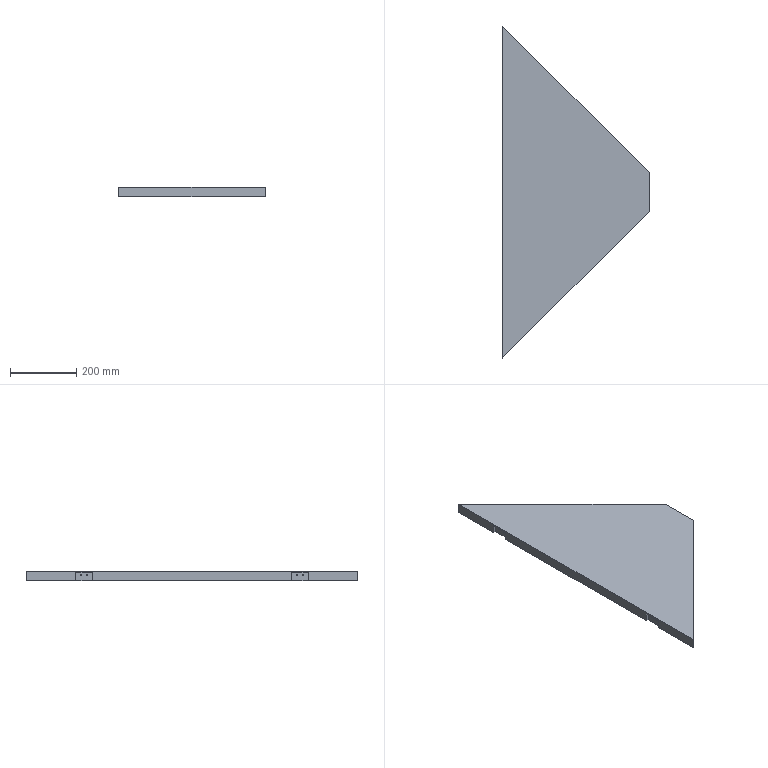Part | SolidWorks | features Cut 1, Extrusion 1, HoleWzd 1, ICE 1, Shell 1 | 1 solid | 35 faces | box 440 x 1000 x 30 mm | volume 2685666 mm3 | plane 27 | cylinder 8 | commonest cylinder face diameters 3.3 x8
STEP:
#1=CARTESIAN_POINT('',(-488.,335.,19.15));
#2=VERTEX_POINT('',#1);
#3=CARTESIAN_POINT('',(-488.,335.,15.85));
#4=VERTEX_POINT('',#3);
#5=CARTESIAN_POINT('',(-488.,335.,17.5));
#6=DIRECTION('',(1.,0.,0.));
#7=DIRECTION('',(0.,0.,-1.));
#8=AXIS2_PLACEMENT_3D('',#5,#6,#7);
#9=CIRCLE('',#8,1.65);
#10=EDGE_CURVE('',#2,#4,#9,.T.);
#11=ORIENTED_EDGE('',*,*,#10,.T.);
#12=CARTESIAN_POINT('',(-493.,335.,15.85));
#13=VERTEX_POINT('',#12);
#14=CARTESIAN_POINT('',(-493.,335.,15.85));
#15=DIRECTION('',(-1.,0.,0.));
#16=VECTOR('',#15,1000.);
#17=LINE('',#14,#16);
#18=EDGE_CURVE('',#4,#13,#17,.T.);
#19=ORIENTED_EDGE('',*,*,#18,.T.);
#20=CARTESIAN_POINT('',(-493.,335.,19.15));
#21=VERTEX_POINT('',#20);
#22=CARTESIAN_POINT('',(-493.,335.,17.5));
#23=DIRECTION('',(-1.,0.,0.));
#24=DIRECTION('',(0.,0.,1.));
#25=AXIS2_PLACEMENT_3D('',#22,#23,#24);
#26=CIRCLE('',#25,1.65);
#27=EDGE_CURVE('',#13,#21,#26,.T.);
#28=ORIENTED_EDGE('',*,*,#27,.T.);
#29=CARTESIAN_POINT('',(-493.,335.,19.15));
#30=DIRECTION('',(-1.,0.,0.));
#31=VECTOR('',#30,1000.);
#32=LINE('',#29,#31);
#33=EDGE_CURVE('',#2,#21,#32,.T.);
#34=ORIENTED_EDGE('',*,*,#33,.F.);
#35=EDGE_LOOP('',(#11,#19,#28,#34));
#36=FACE_OUTER_BOUND('',#35,.T.);
#37=CARTESIAN_POINT('',(-493.,335.,17.5));
#38=DIRECTION('',(-1.,0.,0.));
#39=DIRECTION('',(0.,0.,1.));
#40=AXIS2_PLACEMENT_3D('',#37,#38,#39);
#41=CYLINDRICAL_SURFACE('',#40,1.65);
#42=ADVANCED_FACE('',(#36),#41,.F.);
#43=CARTESIAN_POINT('',(-488.,315.,19.15));
#44=VERTEX_POINT('',#43);
#45=CARTESIAN_POINT('',(-488.,315.,15.85));
#46=VERTEX_POINT('',#45);
#47=CARTESIAN_POINT('',(-488.,315.,17.5));
#48=DIRECTION('',(1.,0.,0.));
#49=DIRECTION('',(0.,0.,-1.));
#50=AXIS2_PLACEMENT_3D('',#47,#48,#49);
#51=CIRCLE('',#50,1.65);
#52=EDGE_CURVE('',#44,#46,#51,.T.);
#53=ORIENTED_EDGE('',*,*,#52,.T.);
#54=CARTESIAN_POINT('',(-493.,315.,15.85));
#55=VERTEX_POINT('',#54);
#56=CARTESIAN_POINT('',(-493.,315.,15.85));
#57=DIRECTION('',(-1.,0.,0.));
#58=VECTOR('',#57,1000.);
#59=LINE('',#56,#58);
#60=EDGE_CURVE('',#46,#55,#59,.T.);
#61=ORIENTED_EDGE('',*,*,#60,.T.);
#62=CARTESIAN_POINT('',(-493.,315.,19.15));
#63=VERTEX_POINT('',#62);
#64=CARTESIAN_POINT('',(-493.,315.,17.5));
#65=DIRECTION('',(-1.,0.,0.));
#66=DIRECTION('',(0.,0.,1.));
#67=AXIS2_PLACEMENT_3D('',#64,#65,#66);
#68=CIRCLE('',#67,1.65);
#69=EDGE_CURVE('',#55,#63,#68,.T.);
#70=ORIENTED_EDGE('',*,*,#69,.T.);
#71=CARTESIAN_POINT('',(-493.,315.,19.15));
#72=DIRECTION('',(-1.,0.,0.));
#73=VECTOR('',#72,1000.);
#74=LINE('',#71,#73);
#75=EDGE_CURVE('',#44,#63,#74,.T.);
#76=ORIENTED_EDGE('',*,*,#75,.F.);
#77=EDGE_LOOP('',(#53,#61,#70,#76));
#78=FACE_OUTER_BOUND('',#77,.T.);
#79=CARTESIAN_POINT('',(-493.,315.,17.5));
#80=DIRECTION('',(-1.,0.,0.));
#81=DIRECTION('',(0.,0.,1.));
#82=AXIS2_PLACEMENT_3D('',#79,#80,#81);
#83=CYLINDRICAL_SURFACE('',#82,1.65);
#84=ADVANCED_FACE('',(#78),#83,.F.);
#85=CARTESIAN_POINT('',(-488.,-315.,19.15));
#86=VERTEX_POINT('',#85);
#87=CARTESIAN_POINT('',(-488.,-315.,15.85));
#88=VERTEX_POINT('',#87);
#89=CARTESIAN_POINT('',(-488.,-315.,17.5));
#90=DIRECTION('',(1.,0.,0.));
#91=DIRECTION('',(0.,0.,-1.));
#92=AXIS2_PLACEMENT_3D('',#89,#90,#91);
#93=CIRCLE('',#92,1.65);
#94=EDGE_CURVE('',#86,#88,#93,.T.);
#95=ORIENTED_EDGE('',*,*,#94,.T.);
#96=CARTESIAN_POINT('',(-493.,-315.,15.85));
#97=VERTEX_POINT('',#96);
#98=CARTESIAN_POINT('',(-493.,-315.,15.85));
#99=DIRECTION('',(-1.,0.,0.));
#100=VECTOR('',#99,1000.);
#101=LINE('',#98,#100);
#102=EDGE_CURVE('',#88,#97,#101,.T.);
#103=ORIENTED_EDGE('',*,*,#102,.T.);
#104=CARTESIAN_POINT('',(-493.,-315.,19.15));
#105=VERTEX_POINT('',#104);
#106=CARTESIAN_POINT('',(-493.,-315.,17.5));
#107=DIRECTION('',(-1.,0.,0.));
#108=DIRECTION('',(0.,0.,1.));
#109=AXIS2_PLACEMENT_3D('',#106,#107,#108);
#110=CIRCLE('',#109,1.65);
#111=EDGE_CURVE('',#97,#105,#110,.T.);
#112=ORIENTED_EDGE('',*,*,#111,.T.);
#113=CARTESIAN_POINT('',(-493.,-315.,19.15));
#114=DIRECTION('',(-1.,0.,0.));
#115=VECTOR('',#114,1000.);
#116=LINE('',#113,#115);
#117=EDGE_CURVE('',#86,#105,#116,.T.);
#118=ORIENTED_EDGE('',*,*,#117,.F.);
#119=EDGE_LOOP('',(#95,#103,#112,#118));
#120=FACE_OUTER_BOUND('',#119,.T.);
#121=CARTESIAN_POINT('',(-493.,-315.,17.5));
#122=DIRECTION('',(-1.,0.,0.));
#123=DIRECTION('',(0.,0.,1.));
#124=AXIS2_PLACEMENT_3D('',#121,#122,#123);
#125=CYLINDRICAL_SURFACE('',#124,1.65);
#126=ADVANCED_FACE('',(#120),#125,.F.);
#127=CARTESIAN_POINT('',(-488.,-335.,19.15));
#128=VERTEX_POINT('',#127);
#129=CARTESIAN_POINT('',(-488.,-335.,15.85));
#130=VERTEX_POINT('',#129);
#131=CARTESIAN_POINT('',(-488.,-335.,17.5));
#132=DIRECTION('',(1.,0.,0.));
#133=DIRECTION('',(0.,0.,-1.));
#134=AXIS2_PLACEMENT_3D('',#131,#132,#133);
#135=CIRCLE('',#134,1.65);
#136=EDGE_CURVE('',#128,#130,#135,.T.);
#137=ORIENTED_EDGE('',*,*,#136,.T.);
#138=CARTESIAN_POINT('',(-493.,-335.,15.85));
#139=VERTEX_POINT('',#138);
#140=CARTESIAN_POINT('',(-493.,-335.,15.85));
#141=DIRECTION('',(-1.,0.,0.));
#142=VECTOR('',#141,1000.);
#143=LINE('',#140,#142);
#144=EDGE_CURVE('',#130,#139,#143,.T.);
#145=ORIENTED_EDGE('',*,*,#144,.T.);
#146=CARTESIAN_POINT('',(-493.,-335.,19.15));
#147=VERTEX_POINT('',#146);
#148=CARTESIAN_POINT('',(-493.,-335.,17.5));
#149=DIRECTION('',(-1.,0.,0.));
#150=DIRECTION('',(0.,0.,1.));
#151=AXIS2_PLACEMENT_3D('',#148,#149,#150);
#152=CIRCLE('',#151,1.65);
#153=EDGE_CURVE('',#139,#147,#152,.T.);
#154=ORIENTED_EDGE('',*,*,#153,.T.);
#155=CARTESIAN_POINT('',(-493.,-335.,19.15));
#156=DIRECTION('',(-1.,0.,0.));
#157=VECTOR('',#156,1000.);
#158=LINE('',#155,#157);
#159=EDGE_CURVE('',#128,#147,#158,.T.);
#160=ORIENTED_EDGE('',*,*,#159,.F.);
#161=EDGE_LOOP('',(#137,#145,#154,#160));
#162=FACE_OUTER_BOUND('',#161,.T.);
#163=CARTESIAN_POINT('',(-493.,-335.,17.5));
#164=DIRECTION('',(-1.,0.,0.));
#165=DIRECTION('',(0.,0.,1.));
#166=AXIS2_PLACEMENT_3D('',#163,#164,#165);
#167=CYLINDRICAL_SURFACE('',#166,1.65);
#168=ADVANCED_FACE('',(#162),#167,.F.);
#169=CARTESIAN_POINT('',(-60.,60.,30.));
#170=VERTEX_POINT('',#169);
#171=CARTESIAN_POINT('',(-60.,-60.,30.));
#172=VERTEX_POINT('',#171);
#173=CARTESIAN_POINT('',(-60.,-60.,30.));
#174=DIRECTION('',(0.,-1.,0.));
#175=VECTOR('',#174,1000.);
#176=LINE('',#173,#175);
#177=EDGE_CURVE('',#170,#172,#176,.T.);
#178=ORIENTED_EDGE('',*,*,#177,.T.);
#179=CARTESIAN_POINT('',(-60.,-60.,0.));
#180=VERTEX_POINT('',#179);
#181=CARTESIAN_POINT('',(-60.,-60.,0.));
#182=DIRECTION('',(0.,0.,1.));
#183=VECTOR('',#182,1000.);
#184=LINE('',#181,#183);
#185=EDGE_CURVE('',#180,#172,#184,.T.);
#186=ORIENTED_EDGE('',*,*,#185,.F.);
#187=CARTESIAN_POINT('',(-60.,60.,0.));
#188=VERTEX_POINT('',#187);
#189=CARTESIAN_POINT('',(-60.,-60.,0.));
#190=DIRECTION('',(0.,-1.,0.));
#191=VECTOR('',#190,1000.);
#192=LINE('',#189,#191);
#193=EDGE_CURVE('',#188,#180,#192,.T.);
#194=ORIENTED_EDGE('',*,*,#193,.F.);
#195=CARTESIAN_POINT('',(-60.,60.,0.));
#196=DIRECTION('',(0.,0.,1.));
#197=VECTOR('',#196,1000.);
#198=LINE('',#195,#197);
#199=EDGE_CURVE('',#188,#170,#198,.T.);
#200=ORIENTED_EDGE('',*,*,#199,.T.);
#201=EDGE_LOOP('',(#178,#186,#194,#200));
#202=FACE_OUTER_BOUND('',#201,.T.);
#203=CARTESIAN_POINT('',(-60.,52.929,25.));
#204=VERTEX_POINT('',#203);
#205=CARTESIAN_POINT('',(-60.,-52.929,25.));
#206=VERTEX_POINT('',#205);
#207=CARTESIAN_POINT('',(-60.,0.,25.));
#208=DIRECTION('',(0.,-1.,0.));
#209=VECTOR('',#208,1000.);
#210=LINE('',#207,#209);
#211=EDGE_CURVE('',#204,#206,#210,.T.);
#212=ORIENTED_EDGE('',*,*,#211,.F.);
#213=CARTESIAN_POINT('',(-60.,52.929,5.));
#214=VERTEX_POINT('',#213);
#215=CARTESIAN_POINT('',(-60.,52.929,0.));
#216=DIRECTION('',(0.,0.,1.));
#217=VECTOR('',#216,1000.);
#218=LINE('',#215,#217);
#219=EDGE_CURVE('',#214,#204,#218,.T.);
#220=ORIENTED_EDGE('',*,*,#219,.F.);
#221=CARTESIAN_POINT('',(-60.,-52.929,5.));
#222=VERTEX_POINT('',#221);
#223=CARTESIAN_POINT('',(-60.,0.,5.));
#224=DIRECTION('',(0.,-1.,0.));
#225=VECTOR('',#224,1000.);
#226=LINE('',#223,#225);
#227=EDGE_CURVE('',#214,#222,#226,.T.);
#228=ORIENTED_EDGE('',*,*,#227,.T.);
#229=CARTESIAN_POINT('',(-60.,-52.929,30.));
#230=DIRECTION('',(0.,0.,1.));
#231=VECTOR('',#230,1000.);
#232=LINE('',#229,#231);
#233=EDGE_CURVE('',#222,#206,#232,.T.);
#234=ORIENTED_EDGE('',*,*,#233,.T.);
#235=EDGE_LOOP('',(#212,#220,#228,#234));
#236=FACE_BOUND('',#235,.T.);
#237=CARTESIAN_POINT('',(-60.,-60.,0.));
#238=DIRECTION('',(-1.,0.,0.));
#239=DIRECTION('',(0.,0.,1.));
#240=AXIS2_PLACEMENT_3D('',#237,#238,#239);
#241=PLANE('',#240);
#242=ADVANCED_FACE('',(#202,#236),#241,.F.);
#243=CARTESIAN_POINT('',(-500.,-500.,0.));
#244=VERTEX_POINT('',#243);
#245=CARTESIAN_POINT('',(0.,0.,0.));
#246=DIRECTION('',(0.7071,0.7071,0.));
#247=VECTOR('',#246,1000.);
#248=LINE('',#245,#247);
#249=EDGE_CURVE('',#244,#180,#248,.T.);
#250=ORIENTED_EDGE('',*,*,#249,.T.);
#251=ORIENTED_EDGE('',*,*,#185,.T.);
#252=CARTESIAN_POINT('',(-500.,-500.,30.));
#253=VERTEX_POINT('',#252);
#254=CARTESIAN_POINT('',(0.,0.,30.));
#255=DIRECTION('',(0.7071,0.7071,0.));
#256=VECTOR('',#255,1000.);
#257=LINE('',#254,#256);
#258=EDGE_CURVE('',#253,#172,#257,.T.);
#259=ORIENTED_EDGE('',*,*,#258,.F.);
#260=CARTESIAN_POINT('',(-500.,-500.,30.));
#261=DIRECTION('',(0.,0.,-1.));
#262=VECTOR('',#261,1000.);
#263=LINE('',#260,#262);
#264=EDGE_CURVE('',#253,#244,#263,.T.);
#265=ORIENTED_EDGE('',*,*,#264,.T.);
#266=EDGE_LOOP('',(#250,#251,#259,#265));
#267=FACE_OUTER_BOUND('',#266,.T.);
#268=CARTESIAN_POINT('',(0.,0.,30.));
#269=DIRECTION('',(-0.7071,0.7071,0.));
#270=DIRECTION('',(-0.7071,-0.7071,0.));
#271=AXIS2_PLACEMENT_3D('',#268,#269,#270);
#272=PLANE('',#271);
#273=ADVANCED_FACE('',(#267),#272,.F.);
#274=CARTESIAN_POINT('',(-500.,500.,30.));
#275=VERTEX_POINT('',#274);
#276=CARTESIAN_POINT('',(-500.,500.,30.));
#277=DIRECTION('',(-0.7071,0.7071,0.));
#278=VECTOR('',#277,1000.);
#279=LINE('',#276,#278);
#280=EDGE_CURVE('',#170,#275,#279,.T.);
#281=ORIENTED_EDGE('',*,*,#280,.F.);
#282=ORIENTED_EDGE('',*,*,#199,.F.);
#283=CARTESIAN_POINT('',(-500.,500.,0.));
#284=VERTEX_POINT('',#283);
#285=CARTESIAN_POINT('',(-500.,500.,0.));
#286=DIRECTION('',(-0.7071,0.7071,0.));
#287=VECTOR('',#286,1000.);
#288=LINE('',#285,#287);
#289=EDGE_CURVE('',#188,#284,#288,.T.);
#290=ORIENTED_EDGE('',*,*,#289,.T.);
#291=CARTESIAN_POINT('',(-500.,500.,30.));
#292=DIRECTION('',(0.,0.,-1.));
#293=VECTOR('',#292,1000.);
#294=LINE('',#291,#293);
#295=EDGE_CURVE('',#275,#284,#294,.T.);
#296=ORIENTED_EDGE('',*,*,#295,.F.);
#297=EDGE_LOOP('',(#281,#282,#290,#296));
#298=FACE_OUTER_BOUND('',#297,.T.);
#299=CARTESIAN_POINT('',(-500.,500.,30.));
#300=DIRECTION('',(-0.7071,-0.7071,0.));
#301=DIRECTION('',(0.7071,-0.7071,0.));
#302=AXIS2_PLACEMENT_3D('',#299,#300,#301);
#303=PLANE('',#302);
#304=ADVANCED_FACE('',(#298),#303,.F.);
#305=CARTESIAN_POINT('',(-500.,300.,25.));
#306=VERTEX_POINT('',#305);
#307=CARTESIAN_POINT('',(-500.,350.,25.));
#308=VERTEX_POINT('',#307);
#309=CARTESIAN_POINT('',(-500.,350.,25.));
#310=DIRECTION('',(0.,1.,0.));
#311=VECTOR('',#310,1000.);
#312=LINE('',#309,#311);
#313=EDGE_CURVE('',#306,#308,#312,.T.);
#314=ORIENTED_EDGE('',*,*,#313,.F.);
#315=CARTESIAN_POINT('',(-500.,300.,0.));
#316=VERTEX_POINT('',#315);
#317=CARTESIAN_POINT('',(-500.,300.,25.));
#318=DIRECTION('',(0.,0.,1.));
#319=VECTOR('',#318,1000.);
#320=LINE('',#317,#319);
#321=EDGE_CURVE('',#316,#306,#320,.T.);
#322=ORIENTED_EDGE('',*,*,#321,.F.);
#323=CARTESIAN_POINT('',(-500.,-300.,0.));
#324=VERTEX_POINT('',#323);
#325=CARTESIAN_POINT('',(-500.,-500.,0.));
#326=DIRECTION('',(0.,-1.,0.));
#327=VECTOR('',#326,1000.);
#328=LINE('',#325,#327);
#329=EDGE_CURVE('',#316,#324,#328,.T.);
#330=ORIENTED_EDGE('',*,*,#329,.T.);
#331=CARTESIAN_POINT('',(-500.,-300.,25.));
#332=VERTEX_POINT('',#331);
#333=CARTESIAN_POINT('',(-500.,-300.,25.));
#334=DIRECTION('',(0.,0.,-1.));
#335=VECTOR('',#334,1000.);
#336=LINE('',#333,#335);
#337=EDGE_CURVE('',#332,#324,#336,.T.);
#338=ORIENTED_EDGE('',*,*,#337,.F.);
#339=CARTESIAN_POINT('',(-500.,-350.,25.));
#340=VERTEX_POINT('',#339);
#341=CARTESIAN_POINT('',(-500.,-350.,25.));
#342=DIRECTION('',(0.,1.,0.));
#343=VECTOR('',#342,1000.);
#344=LINE('',#341,#343);
#345=EDGE_CURVE('',#340,#332,#344,.T.);
#346=ORIENTED_EDGE('',*,*,#345,.F.);
#347=CARTESIAN_POINT('',(-500.,-350.,0.));
#348=VERTEX_POINT('',#347);
#349=CARTESIAN_POINT('',(-500.,-350.,25.));
#350=DIRECTION('',(0.,0.,1.));
#351=VECTOR('',#350,1000.);
#352=LINE('',#349,#351);
#353=EDGE_CURVE('',#348,#340,#352,.T.);
#354=ORIENTED_EDGE('',*,*,#353,.F.);
#355=CARTESIAN_POINT('',(-500.,-500.,0.));
#356=DIRECTION('',(0.,-1.,0.));
#357=VECTOR('',#356,1000.);
#358=LINE('',#355,#357);
#359=EDGE_CURVE('',#348,#244,#358,.T.);
#360=ORIENTED_EDGE('',*,*,#359,.T.);
#361=ORIENTED_EDGE('',*,*,#264,.F.);
#362=CARTESIAN_POINT('',(-500.,-500.,30.));
#363=DIRECTION('',(0.,-1.,0.));
#364=VECTOR('',#363,1000.);
#365=LINE('',#362,#364);
#366=EDGE_CURVE('',#275,#253,#365,.T.);
#367=ORIENTED_EDGE('',*,*,#366,.F.);
#368=ORIENTED_EDGE('',*,*,#295,.T.);
#369=CARTESIAN_POINT('',(-500.,350.,0.));
#370=VERTEX_POINT('',#369);
#371=CARTESIAN_POINT('',(-500.,-500.,0.));
#372=DIRECTION('',(0.,-1.,0.));
#373=VECTOR('',#372,1000.);
#374=LINE('',#371,#373);
#375=EDGE_CURVE('',#284,#370,#374,.T.);
#376=ORIENTED_EDGE('',*,*,#375,.T.);
#377=CARTESIAN_POINT('',(-500.,350.,25.));
#378=DIRECTION('',(0.,0.,-1.));
#379=VECTOR('',#378,1000.);
#380=LINE('',#377,#379);
#381=EDGE_CURVE('',#308,#370,#380,.T.);
#382=ORIENTED_EDGE('',*,*,#381,.F.);
#383=EDGE_LOOP('',(#314,#322,#330,#338,#346,#354,#360,#361,#367,#368,#376,#382));
#384=FACE_OUTER_BOUND('',#383,.T.);
#385=CARTESIAN_POINT('',(-500.,-500.,30.));
#386=DIRECTION('',(1.,0.,0.));
#387=DIRECTION('',(0.,0.,-1.));
#388=AXIS2_PLACEMENT_3D('',#385,#386,#387);
#389=PLANE('',#388);
#390=ADVANCED_FACE('',(#384),#389,.F.);
#391=ORIENTED_EDGE('',*,*,#177,.F.);
#392=ORIENTED_EDGE('',*,*,#280,.T.);
#393=ORIENTED_EDGE('',*,*,#366,.T.);
#394=ORIENTED_EDGE('',*,*,#258,.T.);
#395=EDGE_LOOP('',(#391,#392,#393,#394));
#396=FACE_OUTER_BOUND('',#395,.T.);
#397=CARTESIAN_POINT('',(0.,0.,30.));
#398=DIRECTION('',(0.,0.,1.));
#399=DIRECTION('',(1.,0.,0.));
#400=AXIS2_PLACEMENT_3D('',#397,#398,#399);
#401=PLANE('',#400);
#402=ADVANCED_FACE('',(#396),#401,.T.);
#403=ORIENTED_EDGE('',*,*,#329,.F.);
#404=CARTESIAN_POINT('',(-493.,300.,0.));
#405=VERTEX_POINT('',#404);
#406=CARTESIAN_POINT('',(0.,300.,0.));
#407=DIRECTION('',(1.,0.,0.));
#408=VECTOR('',#407,1000.);
#409=LINE('',#406,#408);
#410=EDGE_CURVE('',#316,#405,#409,.T.);
#411=ORIENTED_EDGE('',*,*,#410,.T.);
#412=CARTESIAN_POINT('',(-493.,350.,0.));
#413=VERTEX_POINT('',#412);
#414=CARTESIAN_POINT('',(-493.,0.,0.));
#415=DIRECTION('',(0.,1.,0.));
#416=VECTOR('',#415,1000.);
#417=LINE('',#414,#416);
#418=EDGE_CURVE('',#405,#413,#417,.T.);
#419=ORIENTED_EDGE('',*,*,#418,.T.);
#420=CARTESIAN_POINT('',(0.,350.,0.));
#421=DIRECTION('',(-1.,0.,0.));
#422=VECTOR('',#421,1000.);
#423=LINE('',#420,#422);
#424=EDGE_CURVE('',#413,#370,#423,.T.);
#425=ORIENTED_EDGE('',*,*,#424,.T.);
#426=ORIENTED_EDGE('',*,*,#375,.F.);
#427=ORIENTED_EDGE('',*,*,#289,.F.);
#428=ORIENTED_EDGE('',*,*,#193,.T.);
#429=ORIENTED_EDGE('',*,*,#249,.F.);
#430=ORIENTED_EDGE('',*,*,#359,.F.);
#431=CARTESIAN_POINT('',(-493.,-350.,0.));
#432=VERTEX_POINT('',#431);
#433=CARTESIAN_POINT('',(0.,-350.,0.));
#434=DIRECTION('',(1.,0.,0.));
#435=VECTOR('',#434,1000.);
#436=LINE('',#433,#435);
#437=EDGE_CURVE('',#348,#432,#436,.T.);
#438=ORIENTED_EDGE('',*,*,#437,.T.);
#439=CARTESIAN_POINT('',(-493.,-300.,0.));
#440=VERTEX_POINT('',#439);
#441=CARTESIAN_POINT('',(-493.,0.,0.));
#442=DIRECTION('',(0.,1.,0.));
#443=VECTOR('',#442,1000.);
#444=LINE('',#441,#443);
#445=EDGE_CURVE('',#432,#440,#444,.T.);
#446=ORIENTED_EDGE('',*,*,#445,.T.);
#447=CARTESIAN_POINT('',(0.,-300.,0.));
#448=DIRECTION('',(-1.,0.,0.));
#449=VECTOR('',#448,1000.);
#450=LINE('',#447,#449);
#451=EDGE_CURVE('',#440,#324,#450,.T.);
#452=ORIENTED_EDGE('',*,*,#451,.T.);
#453=EDGE_LOOP('',(#403,#411,#419,#425,#426,#427,#428,#429,#430,#438,#446,#452));
#454=FACE_OUTER_BOUND('',#453,.T.);
#455=CARTESIAN_POINT('',(0.,0.,0.));
#456=DIRECTION('',(0.,0.,1.));
#457=DIRECTION('',(1.,0.,0.));
#458=AXIS2_PLACEMENT_3D('',#455,#456,#457);
#459=PLANE('',#458);
#460=ADVANCED_FACE('',(#454),#459,.F.);
#461=ORIENTED_EDGE('',*,*,#353,.T.);
#462=CARTESIAN_POINT('',(-493.,-350.,25.));
#463=VERTEX_POINT('',#462);
#464=CARTESIAN_POINT('',(-493.,-350.,25.));
#465=DIRECTION('',(-1.,0.,0.));
#466=VECTOR('',#465,1000.);
#467=LINE('',#464,#466);
#468=EDGE_CURVE('',#463,#340,#467,.T.);
#469=ORIENTED_EDGE('',*,*,#468,.F.);
#470=CARTESIAN_POINT('',(-493.,-350.,25.));
#471=DIRECTION('',(0.,0.,1.));
#472=VECTOR('',#471,1000.);
#473=LINE('',#470,#472);
#474=EDGE_CURVE('',#432,#463,#473,.T.);
#475=ORIENTED_EDGE('',*,*,#474,.F.);
#476=ORIENTED_EDGE('',*,*,#437,.F.);
#477=EDGE_LOOP('',(#461,#469,#475,#476));
#478=FACE_OUTER_BOUND('',#477,.T.);
#479=CARTESIAN_POINT('',(-493.,-350.,25.));
#480=DIRECTION('',(0.,-1.,0.));
#481=DIRECTION('',(0.,0.,-1.));
#482=AXIS2_PLACEMENT_3D('',#479,#480,#481);
#483=PLANE('',#482);
#484=ADVANCED_FACE('',(#478),#483,.F.);
#485=CARTESIAN_POINT('',(-493.,-300.,25.));
#486=VERTEX_POINT('',#485);
#487=CARTESIAN_POINT('',(-493.,-300.,25.));
#488=DIRECTION('',(0.,0.,-1.));
#489=VECTOR('',#488,1000.);
#490=LINE('',#487,#489);
#491=EDGE_CURVE('',#486,#440,#490,.T.);
#492=ORIENTED_EDGE('',*,*,#491,.F.);
#493=CARTESIAN_POINT('',(-493.,-300.,25.));
#494=DIRECTION('',(-1.,0.,0.));
#495=VECTOR('',#494,1000.);
#496=LINE('',#493,#495);
#497=EDGE_CURVE('',#486,#332,#496,.T.);
#498=ORIENTED_EDGE('',*,*,#497,.T.);
#499=ORIENTED_EDGE('',*,*,#337,.T.);
#500=ORIENTED_EDGE('',*,*,#451,.F.);
#501=EDGE_LOOP('',(#492,#498,#499,#500));
#502=FACE_OUTER_BOUND('',#501,.T.);
#503=CARTESIAN_POINT('',(-493.,-300.,25.));
#504=DIRECTION('',(0.,1.,0.));
#505=DIRECTION('',(0.,0.,1.));
#506=AXIS2_PLACEMENT_3D('',#503,#504,#505);
#507=PLANE('',#506);
#508=ADVANCED_FACE('',(#502),#507,.F.);
#509=CARTESIAN_POINT('',(-493.,-315.,17.5));
#510=DIRECTION('',(-1.,0.,0.));
#511=DIRECTION('',(0.,0.,1.));
#512=AXIS2_PLACEMENT_3D('',#509,#510,#511);
#513=CIRCLE('',#512,1.65);
#514=EDGE_CURVE('',#105,#97,#513,.T.);
#515=ORIENTED_EDGE('',*,*,#514,.F.);
#516=ORIENTED_EDGE('',*,*,#111,.F.);
#517=EDGE_LOOP('',(#515,#516));
#518=FACE_BOUND('',#517,.T.);
#519=CARTESIAN_POINT('',(-493.,-335.,17.5));
#520=DIRECTION('',(-1.,0.,0.));
#521=DIRECTION('',(0.,0.,1.));
#522=AXIS2_PLACEMENT_3D('',#519,#520,#521);
#523=CIRCLE('',#522,1.65);
#524=EDGE_CURVE('',#147,#139,#523,.T.);
#525=ORIENTED_EDGE('',*,*,#524,.F.);
#526=ORIENTED_EDGE('',*,*,#153,.F.);
#527=EDGE_LOOP('',(#525,#526));
#528=FACE_BOUND('',#527,.T.);
#529=ORIENTED_EDGE('',*,*,#474,.T.);
#530=CARTESIAN_POINT('',(-493.,-350.,25.));
#531=DIRECTION('',(0.,1.,0.));
#532=VECTOR('',#531,1000.);
#533=LINE('',#530,#532);
#534=EDGE_CURVE('',#463,#486,#533,.T.);
#535=ORIENTED_EDGE('',*,*,#534,.T.);
#536=ORIENTED_EDGE('',*,*,#491,.T.);
#537=ORIENTED_EDGE('',*,*,#445,.F.);
#538=EDGE_LOOP('',(#529,#535,#536,#537));
#539=FACE_OUTER_BOUND('',#538,.T.);
#540=CARTESIAN_POINT('',(-493.,0.,0.));
#541=DIRECTION('',(1.,0.,0.));
#542=DIRECTION('',(0.,0.,-1.));
#543=AXIS2_PLACEMENT_3D('',#540,#541,#542);
#544=PLANE('',#543);
#545=ADVANCED_FACE('',(#518,#528,#539),#544,.F.);
#546=ORIENTED_EDGE('',*,*,#345,.T.);
#547=ORIENTED_EDGE('',*,*,#497,.F.);
#548=ORIENTED_EDGE('',*,*,#534,.F.);
#549=ORIENTED_EDGE('',*,*,#468,.T.);
#550=EDGE_LOOP('',(#546,#547,#548,#549));
#551=FACE_OUTER_BOUND('',#550,.T.);
#552=CARTESIAN_POINT('',(-493.,-350.,25.));
#553=DIRECTION('',(0.,0.,1.));
#554=DIRECTION('',(0.,-1.,0.));
#555=AXIS2_PLACEMENT_3D('',#552,#553,#554);
#556=PLANE('',#555);
#557=ADVANCED_FACE('',(#551),#556,.F.);
#558=ORIENTED_EDGE('',*,*,#321,.T.);
#559=CARTESIAN_POINT('',(-493.,300.,25.));
#560=VERTEX_POINT('',#559);
#561=CARTESIAN_POINT('',(-493.,300.,25.));
#562=DIRECTION('',(-1.,0.,0.));
#563=VECTOR('',#562,1000.);
#564=LINE('',#561,#563);
#565=EDGE_CURVE('',#560,#306,#564,.T.);
#566=ORIENTED_EDGE('',*,*,#565,.F.);
#567=CARTESIAN_POINT('',(-493.,300.,25.));
#568=DIRECTION('',(0.,0.,1.));
#569=VECTOR('',#568,1000.);
#570=LINE('',#567,#569);
#571=EDGE_CURVE('',#405,#560,#570,.T.);
#572=ORIENTED_EDGE('',*,*,#571,.F.);
#573=ORIENTED_EDGE('',*,*,#410,.F.);
#574=EDGE_LOOP('',(#558,#566,#572,#573));
#575=FACE_OUTER_BOUND('',#574,.T.);
#576=CARTESIAN_POINT('',(-493.,300.,25.));
#577=DIRECTION('',(0.,-1.,0.));
#578=DIRECTION('',(0.,0.,-1.));
#579=AXIS2_PLACEMENT_3D('',#576,#577,#578);
#580=PLANE('',#579);
#581=ADVANCED_FACE('',(#575),#580,.F.);
#582=CARTESIAN_POINT('',(-493.,350.,25.));
#583=VERTEX_POINT('',#582);
#584=CARTESIAN_POINT('',(-493.,350.,25.));
#585=DIRECTION('',(0.,0.,-1.));
#586=VECTOR('',#585,1000.);
#587=LINE('',#584,#586);
#588=EDGE_CURVE('',#583,#413,#587,.T.);
#589=ORIENTED_EDGE('',*,*,#588,.F.);
#590=CARTESIAN_POINT('',(-493.,350.,25.));
#591=DIRECTION('',(-1.,0.,0.));
#592=VECTOR('',#591,1000.);
#593=LINE('',#590,#592);
#594=EDGE_CURVE('',#583,#308,#593,.T.);
#595=ORIENTED_EDGE('',*,*,#594,.T.);
#596=ORIENTED_EDGE('',*,*,#381,.T.);
#597=ORIENTED_EDGE('',*,*,#424,.F.);
#598=EDGE_LOOP('',(#589,#595,#596,#597));
#599=FACE_OUTER_BOUND('',#598,.T.);
#600=CARTESIAN_POINT('',(-493.,350.,25.));
#601=DIRECTION('',(0.,1.,0.));
#602=DIRECTION('',(0.,0.,1.));
#603=AXIS2_PLACEMENT_3D('',#600,#601,#602);
#604=PLANE('',#603);
#605=ADVANCED_FACE('',(#599),#604,.F.);
#606=CARTESIAN_POINT('',(-493.,335.,17.5));
#607=DIRECTION('',(-1.,0.,0.));
#608=DIRECTION('',(0.,0.,1.));
#609=AXIS2_PLACEMENT_3D('',#606,#607,#608);
#610=CIRCLE('',#609,1.65);
#611=EDGE_CURVE('',#21,#13,#610,.T.);
#612=ORIENTED_EDGE('',*,*,#611,.F.);
#613=ORIENTED_EDGE('',*,*,#27,.F.);
#614=EDGE_LOOP('',(#612,#613));
#615=FACE_BOUND('',#614,.T.);
#616=CARTESIAN_POINT('',(-493.,315.,17.5));
#617=DIRECTION('',(-1.,0.,0.));
#618=DIRECTION('',(0.,0.,1.));
#619=AXIS2_PLACEMENT_3D('',#616,#617,#618);
#620=CIRCLE('',#619,1.65);
#621=EDGE_CURVE('',#63,#55,#620,.T.);
#622=ORIENTED_EDGE('',*,*,#621,.F.);
#623=ORIENTED_EDGE('',*,*,#69,.F.);
#624=EDGE_LOOP('',(#622,#623));
#625=FACE_BOUND('',#624,.T.);
#626=ORIENTED_EDGE('',*,*,#571,.T.);
#627=CARTESIAN_POINT('',(-493.,350.,25.));
#628=DIRECTION('',(0.,1.,0.));
#629=VECTOR('',#628,1000.);
#630=LINE('',#627,#629);
#631=EDGE_CURVE('',#560,#583,#630,.T.);
#632=ORIENTED_EDGE('',*,*,#631,.T.);
#633=ORIENTED_EDGE('',*,*,#588,.T.);
#634=ORIENTED_EDGE('',*,*,#418,.F.);
#635=EDGE_LOOP('',(#626,#632,#633,#634));
#636=FACE_OUTER_BOUND('',#635,.T.);
#637=CARTESIAN_POINT('',(-493.,0.,0.));
#638=DIRECTION('',(1.,0.,0.));
#639=DIRECTION('',(0.,0.,-1.));
#640=AXIS2_PLACEMENT_3D('',#637,#638,#639);
#641=PLANE('',#640);
#642=ADVANCED_FACE('',(#615,#625,#636),#641,.F.);
#643=ORIENTED_EDGE('',*,*,#313,.T.);
#644=ORIENTED_EDGE('',*,*,#594,.F.);
#645=ORIENTED_EDGE('',*,*,#631,.F.);
#646=ORIENTED_EDGE('',*,*,#565,.T.);
#647=EDGE_LOOP('',(#643,#644,#645,#646));
#648=FACE_OUTER_BOUND('',#647,.T.);
#649=CARTESIAN_POINT('',(-493.,350.,25.));
#650=DIRECTION('',(0.,0.,1.));
#651=DIRECTION('',(0.,-1.,0.));
#652=AXIS2_PLACEMENT_3D('',#649,#650,#651);
#653=PLANE('',#652);
#654=ADVANCED_FACE('',(#648),#653,.F.);
#655=CARTESIAN_POINT('',(-488.,-295.,25.));
#656=VERTEX_POINT('',#655);
#657=CARTESIAN_POINT('',(-495.,-295.,25.));
#658=VERTEX_POINT('',#657);
#659=CARTESIAN_POINT('',(0.,-295.,25.));
#660=DIRECTION('',(-1.,0.,0.));
#661=VECTOR('',#660,1000.);
#662=LINE('',#659,#661);
#663=EDGE_CURVE('',#656,#658,#662,.T.);
#664=ORIENTED_EDGE('',*,*,#663,.T.);
#665=CARTESIAN_POINT('',(-495.,295.,25.));
#666=VERTEX_POINT('',#665);
#667=CARTESIAN_POINT('',(-495.,-500.,25.));
#668=DIRECTION('',(0.,-1.,0.));
#669=VECTOR('',#668,1000.);
#670=LINE('',#667,#669);
#671=EDGE_CURVE('',#666,#658,#670,.T.);
#672=ORIENTED_EDGE('',*,*,#671,.F.);
#673=CARTESIAN_POINT('',(-488.,295.,25.));
#674=VERTEX_POINT('',#673);
#675=CARTESIAN_POINT('',(-493.,295.,25.));
#676=DIRECTION('',(-1.,0.,0.));
#677=VECTOR('',#676,1000.);
#678=LINE('',#675,#677);
#679=EDGE_CURVE('',#674,#666,#678,.T.);
#680=ORIENTED_EDGE('',*,*,#679,.F.);
#681=CARTESIAN_POINT('',(-488.,355.,25.));
#682=VERTEX_POINT('',#681);
#683=CARTESIAN_POINT('',(-488.,0.,25.));
#684=DIRECTION('',(0.,1.,0.));
#685=VECTOR('',#684,1000.);
#686=LINE('',#683,#685);
#687=EDGE_CURVE('',#674,#682,#686,.T.);
#688=ORIENTED_EDGE('',*,*,#687,.T.);
#689=CARTESIAN_POINT('',(-495.,355.,25.));
#690=VERTEX_POINT('',#689);
#691=CARTESIAN_POINT('',(0.,355.,25.));
#692=DIRECTION('',(-1.,0.,0.));
#693=VECTOR('',#692,1000.);
#694=LINE('',#691,#693);
#695=EDGE_CURVE('',#682,#690,#694,.T.);
#696=ORIENTED_EDGE('',*,*,#695,.T.);
#697=CARTESIAN_POINT('',(-495.,487.929,25.));
#698=VERTEX_POINT('',#697);
#699=CARTESIAN_POINT('',(-495.,-500.,25.));
#700=DIRECTION('',(0.,-1.,0.));
#701=VECTOR('',#700,1000.);
#702=LINE('',#699,#701);
#703=EDGE_CURVE('',#698,#690,#702,.T.);
#704=ORIENTED_EDGE('',*,*,#703,.F.);
#705=CARTESIAN_POINT('',(-503.536,496.464,25.));
#706=DIRECTION('',(-0.7071,0.7071,0.));
#707=VECTOR('',#706,1000.);
#708=LINE('',#705,#707);
#709=EDGE_CURVE('',#204,#698,#708,.T.);
#710=ORIENTED_EDGE('',*,*,#709,.F.);
#711=ORIENTED_EDGE('',*,*,#211,.T.);
#712=CARTESIAN_POINT('',(-495.,-487.929,25.));
#713=VERTEX_POINT('',#712);
#714=CARTESIAN_POINT('',(-3.536,3.536,25.));
#715=DIRECTION('',(0.7071,0.7071,0.));
#716=VECTOR('',#715,1000.);
#717=LINE('',#714,#716);
#718=EDGE_CURVE('',#713,#206,#717,.T.);
#719=ORIENTED_EDGE('',*,*,#718,.F.);
#720=CARTESIAN_POINT('',(-495.,-355.,25.));
#721=VERTEX_POINT('',#720);
#722=CARTESIAN_POINT('',(-495.,-500.,25.));
#723=DIRECTION('',(0.,-1.,0.));
#724=VECTOR('',#723,1000.);
#725=LINE('',#722,#724);
#726=EDGE_CURVE('',#721,#713,#725,.T.);
#727=ORIENTED_EDGE('',*,*,#726,.F.);
#728=CARTESIAN_POINT('',(-488.,-355.,25.));
#729=VERTEX_POINT('',#728);
#730=CARTESIAN_POINT('',(-493.,-355.,25.));
#731=DIRECTION('',(-1.,0.,0.));
#732=VECTOR('',#731,1000.);
#733=LINE('',#730,#732);
#734=EDGE_CURVE('',#729,#721,#733,.T.);
#735=ORIENTED_EDGE('',*,*,#734,.F.);
#736=CARTESIAN_POINT('',(-488.,0.,25.));
#737=DIRECTION('',(0.,-1.,0.));
#738=VECTOR('',#737,1000.);
#739=LINE('',#736,#738);
#740=EDGE_CURVE('',#656,#729,#739,.T.);
#741=ORIENTED_EDGE('',*,*,#740,.F.);
#742=EDGE_LOOP('',(#664,#672,#680,#688,#696,#704,#710,#711,#719,#727,#735,#741));
#743=FACE_OUTER_BOUND('',#742,.T.);
#744=CARTESIAN_POINT('',(0.,0.,25.));
#745=DIRECTION('',(0.,0.,1.));
#746=DIRECTION('',(1.,0.,0.));
#747=AXIS2_PLACEMENT_3D('',#744,#745,#746);
#748=PLANE('',#747);
#749=ADVANCED_FACE('',(#743),#748,.F.);
#750=ORIENTED_EDGE('',*,*,#726,.T.);
#751=CARTESIAN_POINT('',(-495.,-487.929,5.));
#752=VERTEX_POINT('',#751);
#753=CARTESIAN_POINT('',(-495.,-487.929,30.));
#754=DIRECTION('',(0.,0.,-1.));
#755=VECTOR('',#754,1000.);
#756=LINE('',#753,#755);
#757=EDGE_CURVE('',#713,#752,#756,.T.);
#758=ORIENTED_EDGE('',*,*,#757,.T.);
#759=CARTESIAN_POINT('',(-495.,-355.,5.));
#760=VERTEX_POINT('',#759);
#761=CARTESIAN_POINT('',(-495.,-500.,5.));
#762=DIRECTION('',(0.,-1.,0.));
#763=VECTOR('',#762,1000.);
#764=LINE('',#761,#763);
#765=EDGE_CURVE('',#760,#752,#764,.T.);
#766=ORIENTED_EDGE('',*,*,#765,.F.);
#767=CARTESIAN_POINT('',(-495.,-355.,25.));
#768=DIRECTION('',(0.,0.,1.));
#769=VECTOR('',#768,1000.);
#770=LINE('',#767,#769);
#771=EDGE_CURVE('',#760,#721,#770,.T.);
#772=ORIENTED_EDGE('',*,*,#771,.T.);
#773=EDGE_LOOP('',(#750,#758,#766,#772));
#774=FACE_OUTER_BOUND('',#773,.T.);
#775=CARTESIAN_POINT('',(-495.,-500.,30.));
#776=DIRECTION('',(1.,0.,0.));
#777=DIRECTION('',(0.,0.,-1.));
#778=AXIS2_PLACEMENT_3D('',#775,#776,#777);
#779=PLANE('',#778);
#780=ADVANCED_FACE('',(#774),#779,.T.);
#781=CARTESIAN_POINT('',(-495.,-295.,5.));
#782=VERTEX_POINT('',#781);
#783=CARTESIAN_POINT('',(-495.,-295.,25.));
#784=DIRECTION('',(0.,0.,-1.));
#785=VECTOR('',#784,1000.);
#786=LINE('',#783,#785);
#787=EDGE_CURVE('',#658,#782,#786,.T.);
#788=ORIENTED_EDGE('',*,*,#787,.T.);
#789=CARTESIAN_POINT('',(-495.,295.,5.));
#790=VERTEX_POINT('',#789);
#791=CARTESIAN_POINT('',(-495.,-500.,5.));
#792=DIRECTION('',(0.,-1.,0.));
#793=VECTOR('',#792,1000.);
#794=LINE('',#791,#793);
#795=EDGE_CURVE('',#790,#782,#794,.T.);
#796=ORIENTED_EDGE('',*,*,#795,.F.);
#797=CARTESIAN_POINT('',(-495.,295.,25.));
#798=DIRECTION('',(0.,0.,1.));
#799=VECTOR('',#798,1000.);
#800=LINE('',#797,#799);
#801=EDGE_CURVE('',#790,#666,#800,.T.);
#802=ORIENTED_EDGE('',*,*,#801,.T.);
#803=ORIENTED_EDGE('',*,*,#671,.T.);
#804=EDGE_LOOP('',(#788,#796,#802,#803));
#805=FACE_OUTER_BOUND('',#804,.T.);
#806=CARTESIAN_POINT('',(-495.,-500.,30.));
#807=DIRECTION('',(1.,0.,0.));
#808=DIRECTION('',(0.,0.,-1.));
#809=AXIS2_PLACEMENT_3D('',#806,#807,#808);
#810=PLANE('',#809);
#811=ADVANCED_FACE('',(#805),#810,.T.);
#812=CARTESIAN_POINT('',(-3.536,3.536,5.));
#813=DIRECTION('',(0.7071,0.7071,0.));
#814=VECTOR('',#813,1000.);
#815=LINE('',#812,#814);
#816=EDGE_CURVE('',#752,#222,#815,.T.);
#817=ORIENTED_EDGE('',*,*,#816,.F.);
#818=ORIENTED_EDGE('',*,*,#757,.F.);
#819=ORIENTED_EDGE('',*,*,#718,.T.);
#820=ORIENTED_EDGE('',*,*,#233,.F.);
#821=EDGE_LOOP('',(#817,#818,#819,#820));
#822=FACE_OUTER_BOUND('',#821,.T.);
#823=CARTESIAN_POINT('',(-3.536,3.536,30.));
#824=DIRECTION('',(-0.7071,0.7071,0.));
#825=DIRECTION('',(-0.7071,-0.7071,0.));
#826=AXIS2_PLACEMENT_3D('',#823,#824,#825);
#827=PLANE('',#826);
#828=ADVANCED_FACE('',(#822),#827,.T.);
#829=ORIENTED_EDGE('',*,*,#709,.T.);
#830=CARTESIAN_POINT('',(-495.,487.929,5.));
#831=VERTEX_POINT('',#830);
#832=CARTESIAN_POINT('',(-495.,487.929,30.));
#833=DIRECTION('',(0.,0.,-1.));
#834=VECTOR('',#833,1000.);
#835=LINE('',#832,#834);
#836=EDGE_CURVE('',#698,#831,#835,.T.);
#837=ORIENTED_EDGE('',*,*,#836,.T.);
#838=CARTESIAN_POINT('',(-503.536,496.464,5.));
#839=DIRECTION('',(-0.7071,0.7071,0.));
#840=VECTOR('',#839,1000.);
#841=LINE('',#838,#840);
#842=EDGE_CURVE('',#214,#831,#841,.T.);
#843=ORIENTED_EDGE('',*,*,#842,.F.);
#844=ORIENTED_EDGE('',*,*,#219,.T.);
#845=EDGE_LOOP('',(#829,#837,#843,#844));
#846=FACE_OUTER_BOUND('',#845,.T.);
#847=CARTESIAN_POINT('',(-503.536,496.464,30.));
#848=DIRECTION('',(-0.7071,-0.7071,0.));
#849=DIRECTION('',(0.7071,-0.7071,0.));
#850=AXIS2_PLACEMENT_3D('',#847,#848,#849);
#851=PLANE('',#850);
#852=ADVANCED_FACE('',(#846),#851,.T.);
#853=CARTESIAN_POINT('',(-495.,355.,5.));
#854=VERTEX_POINT('',#853);
#855=CARTESIAN_POINT('',(-495.,355.,25.));
#856=DIRECTION('',(0.,0.,-1.));
#857=VECTOR('',#856,1000.);
#858=LINE('',#855,#857);
#859=EDGE_CURVE('',#690,#854,#858,.T.);
#860=ORIENTED_EDGE('',*,*,#859,.T.);
#861=CARTESIAN_POINT('',(-495.,-500.,5.));
#862=DIRECTION('',(0.,-1.,0.));
#863=VECTOR('',#862,1000.);
#864=LINE('',#861,#863);
#865=EDGE_CURVE('',#831,#854,#864,.T.);
#866=ORIENTED_EDGE('',*,*,#865,.F.);
#867=ORIENTED_EDGE('',*,*,#836,.F.);
#868=ORIENTED_EDGE('',*,*,#703,.T.);
#869=EDGE_LOOP('',(#860,#866,#867,#868));
#870=FACE_OUTER_BOUND('',#869,.T.);
#871=CARTESIAN_POINT('',(-495.,-500.,30.));
#872=DIRECTION('',(1.,0.,0.));
#873=DIRECTION('',(0.,0.,-1.));
#874=AXIS2_PLACEMENT_3D('',#871,#872,#873);
#875=PLANE('',#874);
#876=ADVANCED_FACE('',(#870),#875,.T.);
#877=ORIENTED_EDGE('',*,*,#795,.T.);
#878=CARTESIAN_POINT('',(-488.,-295.,5.));
#879=VERTEX_POINT('',#878);
#880=CARTESIAN_POINT('',(0.,-295.,5.));
#881=DIRECTION('',(-1.,0.,0.));
#882=VECTOR('',#881,1000.);
#883=LINE('',#880,#882);
#884=EDGE_CURVE('',#879,#782,#883,.T.);
#885=ORIENTED_EDGE('',*,*,#884,.F.);
#886=CARTESIAN_POINT('',(-488.,-355.,5.));
#887=VERTEX_POINT('',#886);
#888=CARTESIAN_POINT('',(-488.,0.,5.));
#889=DIRECTION('',(0.,1.,0.));
#890=VECTOR('',#889,1000.);
#891=LINE('',#888,#890);
#892=EDGE_CURVE('',#887,#879,#891,.T.);
#893=ORIENTED_EDGE('',*,*,#892,.F.);
#894=CARTESIAN_POINT('',(0.,-355.,5.));
#895=DIRECTION('',(1.,0.,0.));
#896=VECTOR('',#895,1000.);
#897=LINE('',#894,#896);
#898=EDGE_CURVE('',#760,#887,#897,.T.);
#899=ORIENTED_EDGE('',*,*,#898,.F.);
#900=ORIENTED_EDGE('',*,*,#765,.T.);
#901=ORIENTED_EDGE('',*,*,#816,.T.);
#902=ORIENTED_EDGE('',*,*,#227,.F.);
#903=ORIENTED_EDGE('',*,*,#842,.T.);
#904=ORIENTED_EDGE('',*,*,#865,.T.);
#905=CARTESIAN_POINT('',(-488.,355.,5.));
#906=VERTEX_POINT('',#905);
#907=CARTESIAN_POINT('',(0.,355.,5.));
#908=DIRECTION('',(-1.,0.,0.));
#909=VECTOR('',#908,1000.);
#910=LINE('',#907,#909);
#911=EDGE_CURVE('',#906,#854,#910,.T.);
#912=ORIENTED_EDGE('',*,*,#911,.F.);
#913=CARTESIAN_POINT('',(-488.,295.,5.));
#914=VERTEX_POINT('',#913);
#915=CARTESIAN_POINT('',(-488.,0.,5.));
#916=DIRECTION('',(0.,1.,0.));
#917=VECTOR('',#916,1000.);
#918=LINE('',#915,#917);
#919=EDGE_CURVE('',#914,#906,#918,.T.);
#920=ORIENTED_EDGE('',*,*,#919,.F.);
#921=CARTESIAN_POINT('',(0.,295.,5.));
#922=DIRECTION('',(1.,0.,0.));
#923=VECTOR('',#922,1000.);
#924=LINE('',#921,#923);
#925=EDGE_CURVE('',#790,#914,#924,.T.);
#926=ORIENTED_EDGE('',*,*,#925,.F.);
#927=EDGE_LOOP('',(#877,#885,#893,#899,#900,#901,#902,#903,#904,#912,#920,#926));
#928=FACE_OUTER_BOUND('',#927,.T.);
#929=CARTESIAN_POINT('',(0.,0.,5.));
#930=DIRECTION('',(0.,0.,1.));
#931=DIRECTION('',(1.,0.,0.));
#932=AXIS2_PLACEMENT_3D('',#929,#930,#931);
#933=PLANE('',#932);
#934=ADVANCED_FACE('',(#928),#933,.T.);
#935=ORIENTED_EDGE('',*,*,#734,.T.);
#936=ORIENTED_EDGE('',*,*,#771,.F.);
#937=ORIENTED_EDGE('',*,*,#898,.T.);
#938=CARTESIAN_POINT('',(-488.,-355.,25.));
#939=DIRECTION('',(0.,0.,1.));
#940=VECTOR('',#939,1000.);
#941=LINE('',#938,#940);
#942=EDGE_CURVE('',#887,#729,#941,.T.);
#943=ORIENTED_EDGE('',*,*,#942,.T.);
#944=EDGE_LOOP('',(#935,#936,#937,#943));
#945=FACE_OUTER_BOUND('',#944,.T.);
#946=CARTESIAN_POINT('',(-493.,-355.,25.));
#947=DIRECTION('',(0.,-1.,0.));
#948=DIRECTION('',(0.,0.,-1.));
#949=AXIS2_PLACEMENT_3D('',#946,#947,#948);
#950=PLANE('',#949);
#951=ADVANCED_FACE('',(#945),#950,.T.);
#952=CARTESIAN_POINT('',(-488.,-295.,25.));
#953=DIRECTION('',(0.,0.,-1.));
#954=VECTOR('',#953,1000.);
#955=LINE('',#952,#954);
#956=EDGE_CURVE('',#656,#879,#955,.T.);
#957=ORIENTED_EDGE('',*,*,#956,.T.);
#958=ORIENTED_EDGE('',*,*,#884,.T.);
#959=ORIENTED_EDGE('',*,*,#787,.F.);
#960=ORIENTED_EDGE('',*,*,#663,.F.);
#961=EDGE_LOOP('',(#957,#958,#959,#960));
#962=FACE_OUTER_BOUND('',#961,.T.);
#963=CARTESIAN_POINT('',(-493.,-295.,25.));
#964=DIRECTION('',(0.,1.,0.));
#965=DIRECTION('',(0.,0.,1.));
#966=AXIS2_PLACEMENT_3D('',#963,#964,#965);
#967=PLANE('',#966);
#968=ADVANCED_FACE('',(#962),#967,.T.);
#969=ORIENTED_EDGE('',*,*,#94,.F.);
#970=CARTESIAN_POINT('',(-488.,-315.,17.5));
#971=DIRECTION('',(1.,0.,0.));
#972=DIRECTION('',(0.,0.,-1.));
#973=AXIS2_PLACEMENT_3D('',#970,#971,#972);
#974=CIRCLE('',#973,1.65);
#975=EDGE_CURVE('',#88,#86,#974,.T.);
#976=ORIENTED_EDGE('',*,*,#975,.F.);
#977=EDGE_LOOP('',(#969,#976));
#978=FACE_BOUND('',#977,.T.);
#979=ORIENTED_EDGE('',*,*,#136,.F.);
#980=CARTESIAN_POINT('',(-488.,-335.,17.5));
#981=DIRECTION('',(1.,0.,0.));
#982=DIRECTION('',(0.,0.,-1.));
#983=AXIS2_PLACEMENT_3D('',#980,#981,#982);
#984=CIRCLE('',#983,1.65);
#985=EDGE_CURVE('',#130,#128,#984,.T.);
#986=ORIENTED_EDGE('',*,*,#985,.F.);
#987=EDGE_LOOP('',(#979,#986));
#988=FACE_BOUND('',#987,.T.);
#989=ORIENTED_EDGE('',*,*,#740,.T.);
#990=ORIENTED_EDGE('',*,*,#942,.F.);
#991=ORIENTED_EDGE('',*,*,#892,.T.);
#992=ORIENTED_EDGE('',*,*,#956,.F.);
#993=EDGE_LOOP('',(#989,#990,#991,#992));
#994=FACE_OUTER_BOUND('',#993,.T.);
#995=CARTESIAN_POINT('',(-488.,0.,0.));
#996=DIRECTION('',(1.,0.,0.));
#997=DIRECTION('',(0.,0.,-1.));
#998=AXIS2_PLACEMENT_3D('',#995,#996,#997);
#999=PLANE('',#998);
#1000=ADVANCED_FACE('',(#978,#988,#994),#999,.T.);
#1001=ORIENTED_EDGE('',*,*,#679,.T.);
#1002=ORIENTED_EDGE('',*,*,#801,.F.);
#1003=ORIENTED_EDGE('',*,*,#925,.T.);
#1004=CARTESIAN_POINT('',(-488.,295.,25.));
#1005=DIRECTION('',(0.,0.,1.));
#1006=VECTOR('',#1005,1000.);
#1007=LINE('',#1004,#1006);
#1008=EDGE_CURVE('',#914,#674,#1007,.T.);
#1009=ORIENTED_EDGE('',*,*,#1008,.T.);
#1010=EDGE_LOOP('',(#1001,#1002,#1003,#1009));
#1011=FACE_OUTER_BOUND('',#1010,.T.);
#1012=CARTESIAN_POINT('',(-493.,295.,25.));
#1013=DIRECTION('',(0.,-1.,0.));
#1014=DIRECTION('',(0.,0.,-1.));
#1015=AXIS2_PLACEMENT_3D('',#1012,#1013,#1014);
#1016=PLANE('',#1015);
#1017=ADVANCED_FACE('',(#1011),#1016,.T.);
#1018=CARTESIAN_POINT('',(-488.,355.,25.));
#1019=DIRECTION('',(0.,0.,-1.));
#1020=VECTOR('',#1019,1000.);
#1021=LINE('',#1018,#1020);
#1022=EDGE_CURVE('',#682,#906,#1021,.T.);
#1023=ORIENTED_EDGE('',*,*,#1022,.T.);
#1024=ORIENTED_EDGE('',*,*,#911,.T.);
#1025=ORIENTED_EDGE('',*,*,#859,.F.);
#1026=ORIENTED_EDGE('',*,*,#695,.F.);
#1027=EDGE_LOOP('',(#1023,#1024,#1025,#1026));
#1028=FACE_OUTER_BOUND('',#1027,.T.);
#1029=CARTESIAN_POINT('',(-493.,355.,25.));
#1030=DIRECTION('',(0.,1.,0.));
#1031=DIRECTION('',(0.,0.,1.));
#1032=AXIS2_PLACEMENT_3D('',#1029,#1030,#1031);
#1033=PLANE('',#1032);
#1034=ADVANCED_FACE('',(#1028),#1033,.T.);
#1035=ORIENTED_EDGE('',*,*,#10,.F.);
#1036=CARTESIAN_POINT('',(-488.,335.,17.5));
#1037=DIRECTION('',(1.,0.,0.));
#1038=DIRECTION('',(0.,0.,-1.));
#1039=AXIS2_PLACEMENT_3D('',#1036,#1037,#1038);
#1040=CIRCLE('',#1039,1.65);
#1041=EDGE_CURVE('',#4,#2,#1040,.T.);
#1042=ORIENTED_EDGE('',*,*,#1041,.F.);
#1043=EDGE_LOOP('',(#1035,#1042));
#1044=FACE_BOUND('',#1043,.T.);
#1045=ORIENTED_EDGE('',*,*,#52,.F.);
#1046=CARTESIAN_POINT('',(-488.,315.,17.5));
#1047=DIRECTION('',(1.,0.,0.));
#1048=DIRECTION('',(0.,0.,-1.));
#1049=AXIS2_PLACEMENT_3D('',#1046,#1047,#1048);
#1050=CIRCLE('',#1049,1.65);
#1051=EDGE_CURVE('',#46,#44,#1050,.T.);
#1052=ORIENTED_EDGE('',*,*,#1051,.F.);
#1053=EDGE_LOOP('',(#1045,#1052));
#1054=FACE_BOUND('',#1053,.T.);
#1055=ORIENTED_EDGE('',*,*,#1008,.F.);
#1056=ORIENTED_EDGE('',*,*,#919,.T.);
#1057=ORIENTED_EDGE('',*,*,#1022,.F.);
#1058=ORIENTED_EDGE('',*,*,#687,.F.);
#1059=EDGE_LOOP('',(#1055,#1056,#1057,#1058));
#1060=FACE_OUTER_BOUND('',#1059,.T.);
#1061=CARTESIAN_POINT('',(-488.,0.,0.));
#1062=DIRECTION('',(1.,0.,0.));
#1063=DIRECTION('',(0.,0.,-1.));
#1064=AXIS2_PLACEMENT_3D('',#1061,#1062,#1063);
#1065=PLANE('',#1064);
#1066=ADVANCED_FACE('',(#1044,#1054,#1060),#1065,.T.);
#1067=ORIENTED_EDGE('',*,*,#144,.F.);
#1068=ORIENTED_EDGE('',*,*,#985,.T.);
#1069=ORIENTED_EDGE('',*,*,#159,.T.);
#1070=ORIENTED_EDGE('',*,*,#524,.T.);
#1071=EDGE_LOOP('',(#1067,#1068,#1069,#1070));
#1072=FACE_OUTER_BOUND('',#1071,.T.);
#1073=CARTESIAN_POINT('',(-493.,-335.,17.5));
#1074=DIRECTION('',(-1.,0.,0.));
#1075=DIRECTION('',(0.,0.,1.));
#1076=AXIS2_PLACEMENT_3D('',#1073,#1074,#1075);
#1077=CYLINDRICAL_SURFACE('',#1076,1.65);
#1078=ADVANCED_FACE('',(#1072),#1077,.F.);
#1079=ORIENTED_EDGE('',*,*,#102,.F.);
#1080=ORIENTED_EDGE('',*,*,#975,.T.);
#1081=ORIENTED_EDGE('',*,*,#117,.T.);
#1082=ORIENTED_EDGE('',*,*,#514,.T.);
#1083=EDGE_LOOP('',(#1079,#1080,#1081,#1082));
#1084=FACE_OUTER_BOUND('',#1083,.T.);
#1085=CARTESIAN_POINT('',(-493.,-315.,17.5));
#1086=DIRECTION('',(-1.,0.,0.));
#1087=DIRECTION('',(0.,0.,1.));
#1088=AXIS2_PLACEMENT_3D('',#1085,#1086,#1087);
#1089=CYLINDRICAL_SURFACE('',#1088,1.65);
#1090=ADVANCED_FACE('',(#1084),#1089,.F.);
#1091=ORIENTED_EDGE('',*,*,#60,.F.);
#1092=ORIENTED_EDGE('',*,*,#1051,.T.);
#1093=ORIENTED_EDGE('',*,*,#75,.T.);
#1094=ORIENTED_EDGE('',*,*,#621,.T.);
#1095=EDGE_LOOP('',(#1091,#1092,#1093,#1094));
#1096=FACE_OUTER_BOUND('',#1095,.T.);
#1097=CARTESIAN_POINT('',(-493.,315.,17.5));
#1098=DIRECTION('',(-1.,0.,0.));
#1099=DIRECTION('',(0.,0.,1.));
#1100=AXIS2_PLACEMENT_3D('',#1097,#1098,#1099);
#1101=CYLINDRICAL_SURFACE('',#1100,1.65);
#1102=ADVANCED_FACE('',(#1096),#1101,.F.);
#1103=ORIENTED_EDGE('',*,*,#18,.F.);
#1104=ORIENTED_EDGE('',*,*,#1041,.T.);
#1105=ORIENTED_EDGE('',*,*,#33,.T.);
#1106=ORIENTED_EDGE('',*,*,#611,.T.);
#1107=EDGE_LOOP('',(#1103,#1104,#1105,#1106));
#1108=FACE_OUTER_BOUND('',#1107,.T.);
#1109=CARTESIAN_POINT('',(-493.,335.,17.5));
#1110=DIRECTION('',(-1.,0.,0.));
#1111=DIRECTION('',(0.,0.,1.));
#1112=AXIS2_PLACEMENT_3D('',#1109,#1110,#1111);
#1113=CYLINDRICAL_SURFACE('',#1112,1.65);
#1114=ADVANCED_FACE('',(#1108),#1113,.F.);
#1115=CLOSED_SHELL('',(#42,#84,#126,#168,#242,#273,#304,#390,#402,#460,#484,#508,#545,#557,#581,#605,#642,#654,#749,#780,#811,#828,#852,#876,#934,#951,#968,#1000,#1017,#1034,#1066,#1078,#1090,#1102,#1114));
#1116=MANIFOLD_SOLID_BREP('',#1115);
#1117=CARTESIAN_POINT('',(0.,0.,0.));
#1118=DIRECTION('',(0.,0.,1.));
#1119=DIRECTION('',(1.,0.,0.));
#1120=AXIS2_PLACEMENT_3D('',#1117,#1118,#1119);
#1121=(LENGTH_UNIT()NAMED_UNIT(*)SI_UNIT(.MILLI.,.METRE.));
#1122=UNCERTAINTY_MEASURE_WITH_UNIT(LENGTH_MEASURE(0.00001),#1121,'','');
#1123=(NAMED_UNIT(*)PLANE_ANGLE_UNIT()SI_UNIT($,.RADIAN.));
#1124=(NAMED_UNIT(*)SI_UNIT($,.STERADIAN.)SOLID_ANGLE_UNIT());
#1125=(GEOMETRIC_REPRESENTATION_CONTEXT(3)GLOBAL_UNCERTAINTY_ASSIGNED_CONTEXT((#1122))GLOBAL_UNIT_ASSIGNED_CONTEXT((#1121,#1123,#1124))REPRESENTATION_CONTEXT('',''));
#1126=ADVANCED_BREP_SHAPE_REPRESENTATION('',(#1116,#1120),#1125);